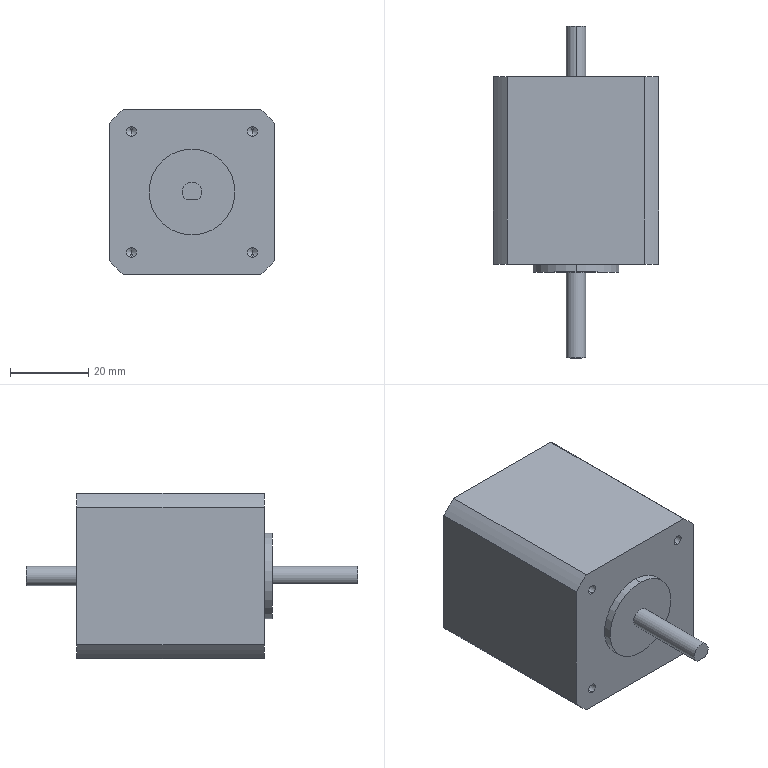Part | NX | features BREP 1 | 1 solid | 35 faces | box 42.3 x 85 x 42.3 mm | volume 86047 mm3 | cylinder 17 | plane 10 | cone 8 | commonest cylinder face diameters 2.5 x8 55 x4 5 x3 22 x2
STEP:
#1=CARTESIAN_POINT('',(1.5,0.,-2.));
#2=VERTEX_POINT('',#1);
#3=CARTESIAN_POINT('',(-1.5,0.,-2.));
#4=VERTEX_POINT('',#3);
#5=CARTESIAN_POINT('',(1.5,0.,-2.));
#6=DIRECTION('',(-1.,0.,0.));
#7=VECTOR('',#6,1000.);
#8=LINE('',#5,#7);
#9=EDGE_CURVE('',#2,#4,#8,.T.);
#10=ORIENTED_EDGE('',*,*,#9,.T.);
#11=CARTESIAN_POINT('',(-1.5,22.,-2.));
#12=VERTEX_POINT('',#11);
#13=CARTESIAN_POINT('',(-1.5,22.,-2.));
#14=DIRECTION('',(0.,-1.,0.));
#15=VECTOR('',#14,1000.);
#16=LINE('',#13,#15);
#17=EDGE_CURVE('',#4,#12,#16,.F.);
#18=ORIENTED_EDGE('',*,*,#17,.T.);
#19=CARTESIAN_POINT('',(1.5,22.,-2.));
#20=VERTEX_POINT('',#19);
#21=CARTESIAN_POINT('',(1.5,22.,-2.));
#22=DIRECTION('',(-1.,0.,0.));
#23=VECTOR('',#22,1000.);
#24=LINE('',#21,#23);
#25=EDGE_CURVE('',#20,#12,#24,.T.);
#26=ORIENTED_EDGE('',*,*,#25,.F.);
#27=CARTESIAN_POINT('',(1.5,22.,-2.));
#28=DIRECTION('',(0.,-1.,0.));
#29=VECTOR('',#28,1000.);
#30=LINE('',#27,#29);
#31=EDGE_CURVE('',#2,#20,#30,.F.);
#32=ORIENTED_EDGE('',*,*,#31,.F.);
#33=EDGE_LOOP('',(#10,#18,#26,#32));
#34=FACE_BOUND('',#33,.T.);
#35=CARTESIAN_POINT('',(1.5,22.,-2.));
#36=DIRECTION('',(0.,0.,1.));
#37=DIRECTION('',(1.,0.,0.));
#38=AXIS2_PLACEMENT_3D('',#35,#36,#37);
#39=PLANE('',#38);
#40=ADVANCED_FACE('',(#34),#39,.F.);
#41=CARTESIAN_POINT('',(-15.5,29.5,-14.25));
#42=VERTEX_POINT('',#41);
#43=CARTESIAN_POINT('',(-15.5,24.,-14.25));
#44=VERTEX_POINT('',#43);
#45=CARTESIAN_POINT('',(-15.5,24.,-14.25));
#46=DIRECTION('',(0.,-1.,0.));
#47=VECTOR('',#46,1000.);
#48=LINE('',#45,#47);
#49=EDGE_CURVE('',#42,#44,#48,.T.);
#50=ORIENTED_EDGE('',*,*,#49,.F.);
#51=CARTESIAN_POINT('',(-15.5,29.5,-16.75));
#52=VERTEX_POINT('',#51);
#53=CARTESIAN_POINT('',(-15.5,29.5,-15.5));
#54=DIRECTION('',(0.,-1.,0.));
#55=DIRECTION('',(0.,0.,-1.));
#56=AXIS2_PLACEMENT_3D('',#53,#54,#55);
#57=CIRCLE('',#56,1.25);
#58=EDGE_CURVE('',#52,#42,#57,.T.);
#59=ORIENTED_EDGE('',*,*,#58,.F.);
#60=CARTESIAN_POINT('',(-15.5,24.,-16.75));
#61=VERTEX_POINT('',#60);
#62=CARTESIAN_POINT('',(-15.5,24.,-16.75));
#63=DIRECTION('',(0.,-1.,0.));
#64=VECTOR('',#63,1000.);
#65=LINE('',#62,#64);
#66=EDGE_CURVE('',#52,#61,#65,.T.);
#67=ORIENTED_EDGE('',*,*,#66,.T.);
#68=CARTESIAN_POINT('',(-15.5,24.,-15.5));
#69=DIRECTION('',(0.,-1.,0.));
#70=DIRECTION('',(0.,0.,-1.));
#71=AXIS2_PLACEMENT_3D('',#68,#69,#70);
#72=CIRCLE('',#71,1.25);
#73=EDGE_CURVE('',#61,#44,#72,.T.);
#74=ORIENTED_EDGE('',*,*,#73,.T.);
#75=EDGE_LOOP('',(#50,#59,#67,#74));
#76=FACE_BOUND('',#75,.T.);
#77=CARTESIAN_POINT('',(-15.5,24.,-15.5));
#78=DIRECTION('',(0.,-1.,0.));
#79=DIRECTION('',(0.,0.,-1.));
#80=AXIS2_PLACEMENT_3D('',#77,#78,#79);
#81=CYLINDRICAL_SURFACE('',#80,1.25);
#82=ADVANCED_FACE('',(#76),#81,.F.);
#83=CARTESIAN_POINT('',(-15.5,30.251,-15.5));
#84=VERTEX_POINT('',#83);
#85=CARTESIAN_POINT('',(-15.5,29.5,-14.25));
#86=DIRECTION('',(0.,-0.515,0.8572));
#87=VECTOR('',#86,1000.);
#88=LINE('',#85,#87);
#89=EDGE_CURVE('',#42,#84,#88,.F.);
#90=ORIENTED_EDGE('',*,*,#89,.T.);
#91=CARTESIAN_POINT('',(-15.5,29.5,-16.75));
#92=DIRECTION('',(0.,-0.515,-0.8572));
#93=VECTOR('',#92,1000.);
#94=LINE('',#91,#93);
#95=EDGE_CURVE('',#52,#84,#94,.F.);
#96=ORIENTED_EDGE('',*,*,#95,.F.);
#97=ORIENTED_EDGE('',*,*,#58,.T.);
#98=EDGE_LOOP('',(#90,#96,#97));
#99=FACE_BOUND('',#98,.T.);
#100=CARTESIAN_POINT('',(-15.5,29.5,-15.5));
#101=DIRECTION('',(0.,-1.,0.));
#102=DIRECTION('',(0.,0.,-1.));
#103=AXIS2_PLACEMENT_3D('',#100,#101,#102);
#104=CONICAL_SURFACE('',#103,1.25,1.03);
#105=ADVANCED_FACE('',(#99),#104,.F.);
#106=CARTESIAN_POINT('',(15.5,29.5,16.75));
#107=VERTEX_POINT('',#106);
#108=CARTESIAN_POINT('',(15.5,24.,16.75));
#109=VERTEX_POINT('',#108);
#110=CARTESIAN_POINT('',(15.5,24.,16.75));
#111=DIRECTION('',(0.,-1.,0.));
#112=VECTOR('',#111,1000.);
#113=LINE('',#110,#112);
#114=EDGE_CURVE('',#107,#109,#113,.T.);
#115=ORIENTED_EDGE('',*,*,#114,.F.);
#116=CARTESIAN_POINT('',(15.5,29.5,14.25));
#117=VERTEX_POINT('',#116);
#118=CARTESIAN_POINT('',(15.5,29.5,15.5));
#119=DIRECTION('',(0.,-1.,0.));
#120=DIRECTION('',(0.,0.,-1.));
#121=AXIS2_PLACEMENT_3D('',#118,#119,#120);
#122=CIRCLE('',#121,1.25);
#123=EDGE_CURVE('',#117,#107,#122,.T.);
#124=ORIENTED_EDGE('',*,*,#123,.F.);
#125=CARTESIAN_POINT('',(15.5,24.,14.25));
#126=VERTEX_POINT('',#125);
#127=CARTESIAN_POINT('',(15.5,24.,14.25));
#128=DIRECTION('',(0.,-1.,0.));
#129=VECTOR('',#128,1000.);
#130=LINE('',#127,#129);
#131=EDGE_CURVE('',#117,#126,#130,.T.);
#132=ORIENTED_EDGE('',*,*,#131,.T.);
#133=CARTESIAN_POINT('',(15.5,24.,15.5));
#134=DIRECTION('',(0.,-1.,0.));
#135=DIRECTION('',(0.,0.,-1.));
#136=AXIS2_PLACEMENT_3D('',#133,#134,#135);
#137=CIRCLE('',#136,1.25);
#138=EDGE_CURVE('',#126,#109,#137,.T.);
#139=ORIENTED_EDGE('',*,*,#138,.T.);
#140=EDGE_LOOP('',(#115,#124,#132,#139));
#141=FACE_BOUND('',#140,.T.);
#142=CARTESIAN_POINT('',(15.5,24.,15.5));
#143=DIRECTION('',(0.,-1.,0.));
#144=DIRECTION('',(0.,0.,-1.));
#145=AXIS2_PLACEMENT_3D('',#142,#143,#144);
#146=CYLINDRICAL_SURFACE('',#145,1.25);
#147=ADVANCED_FACE('',(#141),#146,.F.);
#148=CARTESIAN_POINT('',(15.5,30.251,15.5));
#149=VERTEX_POINT('',#148);
#150=CARTESIAN_POINT('',(15.5,29.5,16.75));
#151=DIRECTION('',(0.,-0.515,0.8572));
#152=VECTOR('',#151,1000.);
#153=LINE('',#150,#152);
#154=EDGE_CURVE('',#107,#149,#153,.F.);
#155=ORIENTED_EDGE('',*,*,#154,.T.);
#156=CARTESIAN_POINT('',(15.5,29.5,14.25));
#157=DIRECTION('',(0.,-0.515,-0.8572));
#158=VECTOR('',#157,1000.);
#159=LINE('',#156,#158);
#160=EDGE_CURVE('',#117,#149,#159,.F.);
#161=ORIENTED_EDGE('',*,*,#160,.F.);
#162=ORIENTED_EDGE('',*,*,#123,.T.);
#163=EDGE_LOOP('',(#155,#161,#162));
#164=FACE_BOUND('',#163,.T.);
#165=CARTESIAN_POINT('',(15.5,29.5,15.5));
#166=DIRECTION('',(0.,-1.,0.));
#167=DIRECTION('',(0.,0.,-1.));
#168=AXIS2_PLACEMENT_3D('',#165,#166,#167);
#169=CONICAL_SURFACE('',#168,1.25,1.03);
#170=ADVANCED_FACE('',(#164),#169,.F.);
#171=CARTESIAN_POINT('',(15.5,29.5,-14.25));
#172=VERTEX_POINT('',#171);
#173=CARTESIAN_POINT('',(15.5,24.,-14.25));
#174=VERTEX_POINT('',#173);
#175=CARTESIAN_POINT('',(15.5,24.,-14.25));
#176=DIRECTION('',(0.,-1.,0.));
#177=VECTOR('',#176,1000.);
#178=LINE('',#175,#177);
#179=EDGE_CURVE('',#172,#174,#178,.T.);
#180=ORIENTED_EDGE('',*,*,#179,.F.);
#181=CARTESIAN_POINT('',(15.5,29.5,-16.75));
#182=VERTEX_POINT('',#181);
#183=CARTESIAN_POINT('',(15.5,29.5,-15.5));
#184=DIRECTION('',(0.,-1.,0.));
#185=DIRECTION('',(0.,0.,-1.));
#186=AXIS2_PLACEMENT_3D('',#183,#184,#185);
#187=CIRCLE('',#186,1.25);
#188=EDGE_CURVE('',#182,#172,#187,.T.);
#189=ORIENTED_EDGE('',*,*,#188,.F.);
#190=CARTESIAN_POINT('',(15.5,24.,-16.75));
#191=VERTEX_POINT('',#190);
#192=CARTESIAN_POINT('',(15.5,24.,-16.75));
#193=DIRECTION('',(0.,-1.,0.));
#194=VECTOR('',#193,1000.);
#195=LINE('',#192,#194);
#196=EDGE_CURVE('',#182,#191,#195,.T.);
#197=ORIENTED_EDGE('',*,*,#196,.T.);
#198=CARTESIAN_POINT('',(15.5,24.,-15.5));
#199=DIRECTION('',(0.,-1.,0.));
#200=DIRECTION('',(0.,0.,-1.));
#201=AXIS2_PLACEMENT_3D('',#198,#199,#200);
#202=CIRCLE('',#201,1.25);
#203=EDGE_CURVE('',#191,#174,#202,.T.);
#204=ORIENTED_EDGE('',*,*,#203,.T.);
#205=EDGE_LOOP('',(#180,#189,#197,#204));
#206=FACE_BOUND('',#205,.T.);
#207=CARTESIAN_POINT('',(15.5,24.,-15.5));
#208=DIRECTION('',(0.,-1.,0.));
#209=DIRECTION('',(0.,0.,-1.));
#210=AXIS2_PLACEMENT_3D('',#207,#208,#209);
#211=CYLINDRICAL_SURFACE('',#210,1.25);
#212=ADVANCED_FACE('',(#206),#211,.F.);
#213=CARTESIAN_POINT('',(15.5,30.251,-15.5));
#214=VERTEX_POINT('',#213);
#215=CARTESIAN_POINT('',(15.5,29.5,-14.25));
#216=DIRECTION('',(0.,-0.515,0.8572));
#217=VECTOR('',#216,1000.);
#218=LINE('',#215,#217);
#219=EDGE_CURVE('',#172,#214,#218,.F.);
#220=ORIENTED_EDGE('',*,*,#219,.T.);
#221=CARTESIAN_POINT('',(15.5,29.5,-16.75));
#222=DIRECTION('',(0.,-0.515,-0.8572));
#223=VECTOR('',#222,1000.);
#224=LINE('',#221,#223);
#225=EDGE_CURVE('',#182,#214,#224,.F.);
#226=ORIENTED_EDGE('',*,*,#225,.F.);
#227=ORIENTED_EDGE('',*,*,#188,.T.);
#228=EDGE_LOOP('',(#220,#226,#227));
#229=FACE_BOUND('',#228,.T.);
#230=CARTESIAN_POINT('',(15.5,29.5,-15.5));
#231=DIRECTION('',(0.,-1.,0.));
#232=DIRECTION('',(0.,0.,-1.));
#233=AXIS2_PLACEMENT_3D('',#230,#231,#232);
#234=CONICAL_SURFACE('',#233,1.25,1.03);
#235=ADVANCED_FACE('',(#229),#234,.F.);
#236=CARTESIAN_POINT('',(-15.5,29.5,16.75));
#237=VERTEX_POINT('',#236);
#238=CARTESIAN_POINT('',(-15.5,24.,16.75));
#239=VERTEX_POINT('',#238);
#240=CARTESIAN_POINT('',(-15.5,24.,16.75));
#241=DIRECTION('',(0.,-1.,0.));
#242=VECTOR('',#241,1000.);
#243=LINE('',#240,#242);
#244=EDGE_CURVE('',#237,#239,#243,.T.);
#245=ORIENTED_EDGE('',*,*,#244,.F.);
#246=CARTESIAN_POINT('',(-15.5,29.5,14.25));
#247=VERTEX_POINT('',#246);
#248=CARTESIAN_POINT('',(-15.5,29.5,15.5));
#249=DIRECTION('',(0.,-1.,0.));
#250=DIRECTION('',(0.,0.,-1.));
#251=AXIS2_PLACEMENT_3D('',#248,#249,#250);
#252=CIRCLE('',#251,1.25);
#253=EDGE_CURVE('',#247,#237,#252,.T.);
#254=ORIENTED_EDGE('',*,*,#253,.F.);
#255=CARTESIAN_POINT('',(-15.5,24.,14.25));
#256=VERTEX_POINT('',#255);
#257=CARTESIAN_POINT('',(-15.5,24.,14.25));
#258=DIRECTION('',(0.,-1.,0.));
#259=VECTOR('',#258,1000.);
#260=LINE('',#257,#259);
#261=EDGE_CURVE('',#247,#256,#260,.T.);
#262=ORIENTED_EDGE('',*,*,#261,.T.);
#263=CARTESIAN_POINT('',(-15.5,24.,15.5));
#264=DIRECTION('',(0.,-1.,0.));
#265=DIRECTION('',(0.,0.,-1.));
#266=AXIS2_PLACEMENT_3D('',#263,#264,#265);
#267=CIRCLE('',#266,1.25);
#268=EDGE_CURVE('',#256,#239,#267,.T.);
#269=ORIENTED_EDGE('',*,*,#268,.T.);
#270=EDGE_LOOP('',(#245,#254,#262,#269));
#271=FACE_BOUND('',#270,.T.);
#272=CARTESIAN_POINT('',(-15.5,24.,15.5));
#273=DIRECTION('',(0.,-1.,0.));
#274=DIRECTION('',(0.,0.,-1.));
#275=AXIS2_PLACEMENT_3D('',#272,#273,#274);
#276=CYLINDRICAL_SURFACE('',#275,1.25);
#277=ADVANCED_FACE('',(#271),#276,.F.);
#278=CARTESIAN_POINT('',(-15.5,30.251,15.5));
#279=VERTEX_POINT('',#278);
#280=CARTESIAN_POINT('',(-15.5,29.5,16.75));
#281=DIRECTION('',(0.,-0.515,0.8572));
#282=VECTOR('',#281,1000.);
#283=LINE('',#280,#282);
#284=EDGE_CURVE('',#237,#279,#283,.F.);
#285=ORIENTED_EDGE('',*,*,#284,.T.);
#286=CARTESIAN_POINT('',(-15.5,29.5,14.25));
#287=DIRECTION('',(0.,-0.515,-0.8572));
#288=VECTOR('',#287,1000.);
#289=LINE('',#286,#288);
#290=EDGE_CURVE('',#247,#279,#289,.F.);
#291=ORIENTED_EDGE('',*,*,#290,.F.);
#292=ORIENTED_EDGE('',*,*,#253,.T.);
#293=EDGE_LOOP('',(#285,#291,#292));
#294=FACE_BOUND('',#293,.T.);
#295=CARTESIAN_POINT('',(-15.5,29.5,15.5));
#296=DIRECTION('',(0.,-1.,0.));
#297=DIRECTION('',(0.,0.,-1.));
#298=AXIS2_PLACEMENT_3D('',#295,#296,#297);
#299=CONICAL_SURFACE('',#298,1.25,1.03);
#300=ADVANCED_FACE('',(#294),#299,.F.);
#301=CARTESIAN_POINT('',(-21.15,72.,-17.576));
#302=VERTEX_POINT('',#301);
#303=CARTESIAN_POINT('',(-21.15,24.,-17.576));
#304=VERTEX_POINT('',#303);
#305=CARTESIAN_POINT('',(-21.15,0.,-17.576));
#306=DIRECTION('',(0.,-1.,0.));
#307=VECTOR('',#306,1000.);
#308=LINE('',#305,#307);
#309=EDGE_CURVE('',#302,#304,#308,.T.);
#310=ORIENTED_EDGE('',*,*,#309,.T.);
#311=CARTESIAN_POINT('',(-21.15,24.,17.576));
#312=VERTEX_POINT('',#311);
#313=CARTESIAN_POINT('',(-21.15,24.,0.));
#314=DIRECTION('',(0.,0.,1.));
#315=VECTOR('',#314,1000.);
#316=LINE('',#313,#315);
#317=EDGE_CURVE('',#304,#312,#316,.T.);
#318=ORIENTED_EDGE('',*,*,#317,.T.);
#319=CARTESIAN_POINT('',(-21.15,72.,17.576));
#320=VERTEX_POINT('',#319);
#321=CARTESIAN_POINT('',(-21.15,0.,17.576));
#322=DIRECTION('',(0.,1.,0.));
#323=VECTOR('',#322,1000.);
#324=LINE('',#321,#323);
#325=EDGE_CURVE('',#312,#320,#324,.T.);
#326=ORIENTED_EDGE('',*,*,#325,.T.);
#327=CARTESIAN_POINT('',(-21.15,72.,0.));
#328=DIRECTION('',(0.,0.,-1.));
#329=VECTOR('',#328,1000.);
#330=LINE('',#327,#329);
#331=EDGE_CURVE('',#320,#302,#330,.T.);
#332=ORIENTED_EDGE('',*,*,#331,.T.);
#333=EDGE_LOOP('',(#310,#318,#326,#332));
#334=FACE_BOUND('',#333,.T.);
#335=CARTESIAN_POINT('',(-21.15,0.,-21.15));
#336=DIRECTION('',(-1.,0.,0.));
#337=DIRECTION('',(0.,0.,1.));
#338=AXIS2_PLACEMENT_3D('',#335,#336,#337);
#339=PLANE('',#338);
#340=ADVANCED_FACE('',(#334),#339,.T.);
#341=CARTESIAN_POINT('',(17.576,72.,-21.15));
#342=VERTEX_POINT('',#341);
#343=CARTESIAN_POINT('',(17.576,24.,-21.15));
#344=VERTEX_POINT('',#343);
#345=CARTESIAN_POINT('',(17.576,0.,-21.15));
#346=DIRECTION('',(0.,-1.,0.));
#347=VECTOR('',#346,1000.);
#348=LINE('',#345,#347);
#349=EDGE_CURVE('',#342,#344,#348,.T.);
#350=ORIENTED_EDGE('',*,*,#349,.T.);
#351=CARTESIAN_POINT('',(-17.576,24.,-21.15));
#352=VERTEX_POINT('',#351);
#353=CARTESIAN_POINT('',(-11.,24.,-21.15));
#354=DIRECTION('',(-1.,0.,0.));
#355=VECTOR('',#354,1000.);
#356=LINE('',#353,#355);
#357=EDGE_CURVE('',#344,#352,#356,.T.);
#358=ORIENTED_EDGE('',*,*,#357,.T.);
#359=CARTESIAN_POINT('',(-17.576,72.,-21.15));
#360=VERTEX_POINT('',#359);
#361=CARTESIAN_POINT('',(-17.576,0.,-21.15));
#362=DIRECTION('',(0.,1.,0.));
#363=VECTOR('',#362,1000.);
#364=LINE('',#361,#363);
#365=EDGE_CURVE('',#352,#360,#364,.T.);
#366=ORIENTED_EDGE('',*,*,#365,.T.);
#367=CARTESIAN_POINT('',(-27.5,72.,-21.15));
#368=DIRECTION('',(1.,0.,0.));
#369=VECTOR('',#368,1000.);
#370=LINE('',#367,#369);
#371=EDGE_CURVE('',#360,#342,#370,.T.);
#372=ORIENTED_EDGE('',*,*,#371,.T.);
#373=EDGE_LOOP('',(#350,#358,#366,#372));
#374=FACE_BOUND('',#373,.T.);
#375=CARTESIAN_POINT('',(21.15,0.,-21.15));
#376=DIRECTION('',(0.,0.,-1.));
#377=DIRECTION('',(-1.,0.,0.));
#378=AXIS2_PLACEMENT_3D('',#375,#376,#377);
#379=PLANE('',#378);
#380=ADVANCED_FACE('',(#374),#379,.T.);
#381=CARTESIAN_POINT('',(21.15,72.,17.576));
#382=VERTEX_POINT('',#381);
#383=CARTESIAN_POINT('',(21.15,24.,17.576));
#384=VERTEX_POINT('',#383);
#385=CARTESIAN_POINT('',(21.15,0.,17.576));
#386=DIRECTION('',(0.,-1.,0.));
#387=VECTOR('',#386,1000.);
#388=LINE('',#385,#387);
#389=EDGE_CURVE('',#382,#384,#388,.T.);
#390=ORIENTED_EDGE('',*,*,#389,.T.);
#391=CARTESIAN_POINT('',(21.15,24.,-17.576));
#392=VERTEX_POINT('',#391);
#393=CARTESIAN_POINT('',(21.15,24.,0.));
#394=DIRECTION('',(0.,0.,-1.));
#395=VECTOR('',#394,1000.);
#396=LINE('',#393,#395);
#397=EDGE_CURVE('',#384,#392,#396,.T.);
#398=ORIENTED_EDGE('',*,*,#397,.T.);
#399=CARTESIAN_POINT('',(21.15,72.,-17.576));
#400=VERTEX_POINT('',#399);
#401=CARTESIAN_POINT('',(21.15,0.,-17.576));
#402=DIRECTION('',(0.,1.,0.));
#403=VECTOR('',#402,1000.);
#404=LINE('',#401,#403);
#405=EDGE_CURVE('',#392,#400,#404,.T.);
#406=ORIENTED_EDGE('',*,*,#405,.T.);
#407=CARTESIAN_POINT('',(21.15,72.,0.));
#408=DIRECTION('',(0.,0.,1.));
#409=VECTOR('',#408,1000.);
#410=LINE('',#407,#409);
#411=EDGE_CURVE('',#400,#382,#410,.T.);
#412=ORIENTED_EDGE('',*,*,#411,.T.);
#413=EDGE_LOOP('',(#390,#398,#406,#412));
#414=FACE_BOUND('',#413,.T.);
#415=CARTESIAN_POINT('',(21.15,0.,-21.15));
#416=DIRECTION('',(1.,0.,0.));
#417=DIRECTION('',(0.,0.,-1.));
#418=AXIS2_PLACEMENT_3D('',#415,#416,#417);
#419=PLANE('',#418);
#420=ADVANCED_FACE('',(#414),#419,.T.);
#421=CARTESIAN_POINT('',(-17.576,72.,21.15));
#422=VERTEX_POINT('',#421);
#423=CARTESIAN_POINT('',(-17.576,24.,21.15));
#424=VERTEX_POINT('',#423);
#425=CARTESIAN_POINT('',(-17.576,0.,21.15));
#426=DIRECTION('',(0.,-1.,0.));
#427=VECTOR('',#426,1000.);
#428=LINE('',#425,#427);
#429=EDGE_CURVE('',#422,#424,#428,.T.);
#430=ORIENTED_EDGE('',*,*,#429,.T.);
#431=CARTESIAN_POINT('',(17.576,24.,21.15));
#432=VERTEX_POINT('',#431);
#433=CARTESIAN_POINT('',(-11.,24.,21.15));
#434=DIRECTION('',(1.,0.,0.));
#435=VECTOR('',#434,1000.);
#436=LINE('',#433,#435);
#437=EDGE_CURVE('',#424,#432,#436,.T.);
#438=ORIENTED_EDGE('',*,*,#437,.T.);
#439=CARTESIAN_POINT('',(17.576,72.,21.15));
#440=VERTEX_POINT('',#439);
#441=CARTESIAN_POINT('',(17.576,0.,21.15));
#442=DIRECTION('',(0.,1.,0.));
#443=VECTOR('',#442,1000.);
#444=LINE('',#441,#443);
#445=EDGE_CURVE('',#432,#440,#444,.T.);
#446=ORIENTED_EDGE('',*,*,#445,.T.);
#447=CARTESIAN_POINT('',(-27.5,72.,21.15));
#448=DIRECTION('',(-1.,0.,0.));
#449=VECTOR('',#448,1000.);
#450=LINE('',#447,#449);
#451=EDGE_CURVE('',#440,#422,#450,.T.);
#452=ORIENTED_EDGE('',*,*,#451,.T.);
#453=EDGE_LOOP('',(#430,#438,#446,#452));
#454=FACE_BOUND('',#453,.T.);
#455=CARTESIAN_POINT('',(21.15,0.,21.15));
#456=DIRECTION('',(0.,0.,1.));
#457=DIRECTION('',(1.,0.,0.));
#458=AXIS2_PLACEMENT_3D('',#455,#456,#457);
#459=PLANE('',#458);
#460=ADVANCED_FACE('',(#454),#459,.T.);
#461=CARTESIAN_POINT('',(0.,85.,-2.5));
#462=VERTEX_POINT('',#461);
#463=CARTESIAN_POINT('',(0.,85.,2.5));
#464=VERTEX_POINT('',#463);
#465=CARTESIAN_POINT('',(0.,85.,0.));
#466=DIRECTION('',(0.,-1.,0.));
#467=DIRECTION('',(0.,0.,-1.));
#468=AXIS2_PLACEMENT_3D('',#465,#466,#467);
#469=CIRCLE('',#468,2.5);
#470=EDGE_CURVE('',#462,#464,#469,.T.);
#471=ORIENTED_EDGE('',*,*,#470,.F.);
#472=CARTESIAN_POINT('',(0.,85.,0.));
#473=DIRECTION('',(0.,-1.,0.));
#474=DIRECTION('',(0.,0.,-1.));
#475=AXIS2_PLACEMENT_3D('',#472,#473,#474);
#476=CIRCLE('',#475,2.5);
#477=EDGE_CURVE('',#464,#462,#476,.T.);
#478=ORIENTED_EDGE('',*,*,#477,.F.);
#479=EDGE_LOOP('',(#471,#478));
#480=FACE_BOUND('',#479,.T.);
#481=CARTESIAN_POINT('',(-2.5,85.,0.));
#482=DIRECTION('',(0.,-1.,0.));
#483=DIRECTION('',(0.,0.,-1.));
#484=AXIS2_PLACEMENT_3D('',#481,#482,#483);
#485=PLANE('',#484);
#486=ADVANCED_FACE('',(#480),#485,.F.);
#487=CARTESIAN_POINT('',(0.,72.,2.5));
#488=VERTEX_POINT('',#487);
#489=CARTESIAN_POINT('',(0.,0.,2.5));
#490=DIRECTION('',(0.,-1.,0.));
#491=VECTOR('',#490,1000.);
#492=LINE('',#489,#491);
#493=EDGE_CURVE('',#464,#488,#492,.T.);
#494=ORIENTED_EDGE('',*,*,#493,.F.);
#495=ORIENTED_EDGE('',*,*,#477,.T.);
#496=CARTESIAN_POINT('',(0.,72.,-2.5));
#497=VERTEX_POINT('',#496);
#498=CARTESIAN_POINT('',(0.,0.,-2.5));
#499=DIRECTION('',(0.,-1.,0.));
#500=VECTOR('',#499,1000.);
#501=LINE('',#498,#500);
#502=EDGE_CURVE('',#462,#497,#501,.T.);
#503=ORIENTED_EDGE('',*,*,#502,.T.);
#504=CARTESIAN_POINT('',(0.,72.,0.));
#505=DIRECTION('',(0.,-1.,0.));
#506=DIRECTION('',(0.,0.,-1.));
#507=AXIS2_PLACEMENT_3D('',#504,#505,#506);
#508=CIRCLE('',#507,2.5);
#509=EDGE_CURVE('',#488,#497,#508,.T.);
#510=ORIENTED_EDGE('',*,*,#509,.F.);
#511=EDGE_LOOP('',(#494,#495,#503,#510));
#512=FACE_BOUND('',#511,.T.);
#513=CARTESIAN_POINT('',(0.,0.,0.));
#514=DIRECTION('',(0.,-1.,0.));
#515=DIRECTION('',(0.,0.,-1.));
#516=AXIS2_PLACEMENT_3D('',#513,#514,#515);
#517=CYLINDRICAL_SURFACE('',#516,2.5);
#518=ADVANCED_FACE('',(#512),#517,.T.);
#519=CARTESIAN_POINT('',(0.,24.,11.));
#520=VERTEX_POINT('',#519);
#521=CARTESIAN_POINT('',(0.,22.,11.));
#522=VERTEX_POINT('',#521);
#523=CARTESIAN_POINT('',(0.,0.,11.));
#524=DIRECTION('',(0.,-1.,0.));
#525=VECTOR('',#524,1000.);
#526=LINE('',#523,#525);
#527=EDGE_CURVE('',#520,#522,#526,.T.);
#528=ORIENTED_EDGE('',*,*,#527,.F.);
#529=CARTESIAN_POINT('',(0.,24.,-11.));
#530=VERTEX_POINT('',#529);
#531=CARTESIAN_POINT('',(0.,24.,0.));
#532=DIRECTION('',(0.,-1.,0.));
#533=DIRECTION('',(0.,0.,-1.));
#534=AXIS2_PLACEMENT_3D('',#531,#532,#533);
#535=CIRCLE('',#534,11.);
#536=EDGE_CURVE('',#520,#530,#535,.T.);
#537=ORIENTED_EDGE('',*,*,#536,.T.);
#538=CARTESIAN_POINT('',(0.,22.,-11.));
#539=VERTEX_POINT('',#538);
#540=CARTESIAN_POINT('',(0.,0.,-11.));
#541=DIRECTION('',(0.,-1.,0.));
#542=VECTOR('',#541,1000.);
#543=LINE('',#540,#542);
#544=EDGE_CURVE('',#530,#539,#543,.T.);
#545=ORIENTED_EDGE('',*,*,#544,.T.);
#546=CARTESIAN_POINT('',(0.,22.,0.));
#547=DIRECTION('',(0.,-1.,0.));
#548=DIRECTION('',(0.,0.,-1.));
#549=AXIS2_PLACEMENT_3D('',#546,#547,#548);
#550=CIRCLE('',#549,11.);
#551=EDGE_CURVE('',#522,#539,#550,.T.);
#552=ORIENTED_EDGE('',*,*,#551,.F.);
#553=EDGE_LOOP('',(#528,#537,#545,#552));
#554=FACE_BOUND('',#553,.T.);
#555=CARTESIAN_POINT('',(0.,0.,0.));
#556=DIRECTION('',(0.,-1.,0.));
#557=DIRECTION('',(0.,0.,-1.));
#558=AXIS2_PLACEMENT_3D('',#555,#556,#557);
#559=CYLINDRICAL_SURFACE('',#558,11.);
#560=ADVANCED_FACE('',(#554),#559,.T.);
#561=CARTESIAN_POINT('',(0.,22.,0.));
#562=DIRECTION('',(0.,-1.,0.));
#563=DIRECTION('',(0.,0.,-1.));
#564=AXIS2_PLACEMENT_3D('',#561,#562,#563);
#565=CIRCLE('',#564,11.);
#566=EDGE_CURVE('',#539,#522,#565,.T.);
#567=ORIENTED_EDGE('',*,*,#566,.T.);
#568=ORIENTED_EDGE('',*,*,#551,.T.);
#569=EDGE_LOOP('',(#567,#568));
#570=FACE_BOUND('',#569,.T.);
#571=CARTESIAN_POINT('',(0.,22.,0.));
#572=DIRECTION('',(0.,-1.,0.));
#573=DIRECTION('',(0.,0.,-1.));
#574=AXIS2_PLACEMENT_3D('',#571,#572,#573);
#575=CIRCLE('',#574,2.5);
#576=EDGE_CURVE('',#20,#12,#575,.T.);
#577=ORIENTED_EDGE('',*,*,#576,.F.);
#578=ORIENTED_EDGE('',*,*,#25,.T.);
#579=EDGE_LOOP('',(#577,#578));
#580=FACE_BOUND('',#579,.T.);
#581=CARTESIAN_POINT('',(-2.5,22.,0.));
#582=DIRECTION('',(0.,1.,0.));
#583=DIRECTION('',(0.,0.,1.));
#584=AXIS2_PLACEMENT_3D('',#581,#582,#583);
#585=PLANE('',#584);
#586=ADVANCED_FACE('',(#570,#580),#585,.F.);
#587=ORIENTED_EDGE('',*,*,#576,.T.);
#588=ORIENTED_EDGE('',*,*,#17,.F.);
#589=CARTESIAN_POINT('',(0.,0.,0.));
#590=DIRECTION('',(0.,-1.,0.));
#591=DIRECTION('',(0.,0.,-1.));
#592=AXIS2_PLACEMENT_3D('',#589,#590,#591);
#593=CIRCLE('',#592,2.5);
#594=EDGE_CURVE('',#2,#4,#593,.T.);
#595=ORIENTED_EDGE('',*,*,#594,.F.);
#596=ORIENTED_EDGE('',*,*,#31,.T.);
#597=EDGE_LOOP('',(#587,#588,#595,#596));
#598=FACE_BOUND('',#597,.T.);
#599=CARTESIAN_POINT('',(0.,0.,0.));
#600=DIRECTION('',(0.,-1.,0.));
#601=DIRECTION('',(0.,0.,-1.));
#602=AXIS2_PLACEMENT_3D('',#599,#600,#601);
#603=CYLINDRICAL_SURFACE('',#602,2.5);
#604=ADVANCED_FACE('',(#598),#603,.T.);
#605=ORIENTED_EDGE('',*,*,#594,.T.);
#606=ORIENTED_EDGE('',*,*,#9,.F.);
#607=EDGE_LOOP('',(#605,#606));
#608=FACE_BOUND('',#607,.T.);
#609=CARTESIAN_POINT('',(0.,0.,0.));
#610=DIRECTION('',(0.,1.,0.));
#611=DIRECTION('',(0.,0.,1.));
#612=AXIS2_PLACEMENT_3D('',#609,#610,#611);
#613=PLANE('',#612);
#614=ADVANCED_FACE('',(#608),#613,.F.);
#615=ORIENTED_EDGE('',*,*,#331,.F.);
#616=CARTESIAN_POINT('',(0.,72.,0.));
#617=DIRECTION('',(0.,-1.,0.));
#618=DIRECTION('',(0.,0.,-1.));
#619=AXIS2_PLACEMENT_3D('',#616,#617,#618);
#620=CIRCLE('',#619,27.5);
#621=EDGE_CURVE('',#422,#320,#620,.T.);
#622=ORIENTED_EDGE('',*,*,#621,.F.);
#623=ORIENTED_EDGE('',*,*,#451,.F.);
#624=CARTESIAN_POINT('',(0.,72.,0.));
#625=DIRECTION('',(0.,-1.,0.));
#626=DIRECTION('',(0.,0.,-1.));
#627=AXIS2_PLACEMENT_3D('',#624,#625,#626);
#628=CIRCLE('',#627,27.5);
#629=EDGE_CURVE('',#382,#440,#628,.T.);
#630=ORIENTED_EDGE('',*,*,#629,.F.);
#631=ORIENTED_EDGE('',*,*,#411,.F.);
#632=CARTESIAN_POINT('',(0.,72.,0.));
#633=DIRECTION('',(0.,-1.,0.));
#634=DIRECTION('',(0.,0.,-1.));
#635=AXIS2_PLACEMENT_3D('',#632,#633,#634);
#636=CIRCLE('',#635,27.5);
#637=EDGE_CURVE('',#342,#400,#636,.T.);
#638=ORIENTED_EDGE('',*,*,#637,.F.);
#639=ORIENTED_EDGE('',*,*,#371,.F.);
#640=CARTESIAN_POINT('',(0.,72.,0.));
#641=DIRECTION('',(0.,-1.,0.));
#642=DIRECTION('',(0.,0.,-1.));
#643=AXIS2_PLACEMENT_3D('',#640,#641,#642);
#644=CIRCLE('',#643,27.5);
#645=EDGE_CURVE('',#302,#360,#644,.T.);
#646=ORIENTED_EDGE('',*,*,#645,.F.);
#647=EDGE_LOOP('',(#615,#622,#623,#630,#631,#638,#639,#646));
#648=FACE_BOUND('',#647,.T.);
#649=CARTESIAN_POINT('',(0.,72.,0.));
#650=DIRECTION('',(0.,-1.,0.));
#651=DIRECTION('',(0.,0.,-1.));
#652=AXIS2_PLACEMENT_3D('',#649,#650,#651);
#653=CIRCLE('',#652,2.5);
#654=EDGE_CURVE('',#497,#488,#653,.T.);
#655=ORIENTED_EDGE('',*,*,#654,.T.);
#656=ORIENTED_EDGE('',*,*,#509,.T.);
#657=EDGE_LOOP('',(#655,#656));
#658=FACE_BOUND('',#657,.T.);
#659=CARTESIAN_POINT('',(-27.5,72.,0.));
#660=DIRECTION('',(0.,-1.,0.));
#661=DIRECTION('',(0.,0.,-1.));
#662=AXIS2_PLACEMENT_3D('',#659,#660,#661);
#663=PLANE('',#662);
#664=ADVANCED_FACE('',(#648,#658),#663,.F.);
#665=ORIENTED_EDGE('',*,*,#389,.F.);
#666=ORIENTED_EDGE('',*,*,#629,.T.);
#667=ORIENTED_EDGE('',*,*,#445,.F.);
#668=CARTESIAN_POINT('',(0.,24.,0.));
#669=DIRECTION('',(0.,-1.,0.));
#670=DIRECTION('',(0.,0.,-1.));
#671=AXIS2_PLACEMENT_3D('',#668,#669,#670);
#672=CIRCLE('',#671,27.5);
#673=EDGE_CURVE('',#384,#432,#672,.T.);
#674=ORIENTED_EDGE('',*,*,#673,.F.);
#675=EDGE_LOOP('',(#665,#666,#667,#674));
#676=FACE_BOUND('',#675,.T.);
#677=CARTESIAN_POINT('',(0.,0.,0.));
#678=DIRECTION('',(0.,-1.,0.));
#679=DIRECTION('',(0.,0.,-1.));
#680=AXIS2_PLACEMENT_3D('',#677,#678,#679);
#681=CYLINDRICAL_SURFACE('',#680,27.5);
#682=ADVANCED_FACE('',(#676),#681,.T.);
#683=ORIENTED_EDGE('',*,*,#349,.F.);
#684=ORIENTED_EDGE('',*,*,#637,.T.);
#685=ORIENTED_EDGE('',*,*,#405,.F.);
#686=CARTESIAN_POINT('',(0.,24.,0.));
#687=DIRECTION('',(0.,-1.,0.));
#688=DIRECTION('',(0.,0.,-1.));
#689=AXIS2_PLACEMENT_3D('',#686,#687,#688);
#690=CIRCLE('',#689,27.5);
#691=EDGE_CURVE('',#344,#392,#690,.T.);
#692=ORIENTED_EDGE('',*,*,#691,.F.);
#693=EDGE_LOOP('',(#683,#684,#685,#692));
#694=FACE_BOUND('',#693,.T.);
#695=CARTESIAN_POINT('',(0.,0.,0.));
#696=DIRECTION('',(0.,-1.,0.));
#697=DIRECTION('',(0.,0.,-1.));
#698=AXIS2_PLACEMENT_3D('',#695,#696,#697);
#699=CYLINDRICAL_SURFACE('',#698,27.5);
#700=ADVANCED_FACE('',(#694),#699,.T.);
#701=ORIENTED_EDGE('',*,*,#325,.F.);
#702=CARTESIAN_POINT('',(0.,24.,0.));
#703=DIRECTION('',(0.,-1.,0.));
#704=DIRECTION('',(0.,0.,-1.));
#705=AXIS2_PLACEMENT_3D('',#702,#703,#704);
#706=CIRCLE('',#705,27.5);
#707=EDGE_CURVE('',#424,#312,#706,.T.);
#708=ORIENTED_EDGE('',*,*,#707,.F.);
#709=ORIENTED_EDGE('',*,*,#429,.F.);
#710=ORIENTED_EDGE('',*,*,#621,.T.);
#711=EDGE_LOOP('',(#701,#708,#709,#710));
#712=FACE_BOUND('',#711,.T.);
#713=CARTESIAN_POINT('',(0.,0.,0.));
#714=DIRECTION('',(0.,-1.,0.));
#715=DIRECTION('',(0.,0.,-1.));
#716=AXIS2_PLACEMENT_3D('',#713,#714,#715);
#717=CYLINDRICAL_SURFACE('',#716,27.5);
#718=ADVANCED_FACE('',(#712),#717,.T.);
#719=ORIENTED_EDGE('',*,*,#309,.F.);
#720=ORIENTED_EDGE('',*,*,#645,.T.);
#721=ORIENTED_EDGE('',*,*,#365,.F.);
#722=CARTESIAN_POINT('',(0.,24.,0.));
#723=DIRECTION('',(0.,-1.,0.));
#724=DIRECTION('',(0.,0.,-1.));
#725=AXIS2_PLACEMENT_3D('',#722,#723,#724);
#726=CIRCLE('',#725,27.5);
#727=EDGE_CURVE('',#304,#352,#726,.T.);
#728=ORIENTED_EDGE('',*,*,#727,.F.);
#729=EDGE_LOOP('',(#719,#720,#721,#728));
#730=FACE_BOUND('',#729,.T.);
#731=CARTESIAN_POINT('',(0.,0.,0.));
#732=DIRECTION('',(0.,-1.,0.));
#733=DIRECTION('',(0.,0.,-1.));
#734=AXIS2_PLACEMENT_3D('',#731,#732,#733);
#735=CYLINDRICAL_SURFACE('',#734,27.5);
#736=ADVANCED_FACE('',(#730),#735,.T.);
#737=ORIENTED_EDGE('',*,*,#317,.F.);
#738=ORIENTED_EDGE('',*,*,#727,.T.);
#739=ORIENTED_EDGE('',*,*,#357,.F.);
#740=ORIENTED_EDGE('',*,*,#691,.T.);
#741=ORIENTED_EDGE('',*,*,#397,.F.);
#742=ORIENTED_EDGE('',*,*,#673,.T.);
#743=ORIENTED_EDGE('',*,*,#437,.F.);
#744=ORIENTED_EDGE('',*,*,#707,.T.);
#745=EDGE_LOOP('',(#737,#738,#739,#740,#741,#742,#743,#744));
#746=FACE_BOUND('',#745,.T.);
#747=CARTESIAN_POINT('',(0.,24.,0.));
#748=DIRECTION('',(0.,-1.,0.));
#749=DIRECTION('',(0.,0.,-1.));
#750=AXIS2_PLACEMENT_3D('',#747,#748,#749);
#751=CIRCLE('',#750,11.);
#752=EDGE_CURVE('',#530,#520,#751,.T.);
#753=ORIENTED_EDGE('',*,*,#752,.F.);
#754=ORIENTED_EDGE('',*,*,#536,.F.);
#755=EDGE_LOOP('',(#753,#754));
#756=FACE_BOUND('',#755,.T.);
#757=ORIENTED_EDGE('',*,*,#268,.F.);
#758=CARTESIAN_POINT('',(-15.5,24.,15.5));
#759=DIRECTION('',(0.,-1.,0.));
#760=DIRECTION('',(0.,0.,-1.));
#761=AXIS2_PLACEMENT_3D('',#758,#759,#760);
#762=CIRCLE('',#761,1.25);
#763=EDGE_CURVE('',#239,#256,#762,.T.);
#764=ORIENTED_EDGE('',*,*,#763,.F.);
#765=EDGE_LOOP('',(#757,#764));
#766=FACE_BOUND('',#765,.T.);
#767=ORIENTED_EDGE('',*,*,#203,.F.);
#768=CARTESIAN_POINT('',(15.5,24.,-15.5));
#769=DIRECTION('',(0.,-1.,0.));
#770=DIRECTION('',(0.,0.,-1.));
#771=AXIS2_PLACEMENT_3D('',#768,#769,#770);
#772=CIRCLE('',#771,1.25);
#773=EDGE_CURVE('',#174,#191,#772,.T.);
#774=ORIENTED_EDGE('',*,*,#773,.F.);
#775=EDGE_LOOP('',(#767,#774));
#776=FACE_BOUND('',#775,.T.);
#777=ORIENTED_EDGE('',*,*,#138,.F.);
#778=CARTESIAN_POINT('',(15.5,24.,15.5));
#779=DIRECTION('',(0.,-1.,0.));
#780=DIRECTION('',(0.,0.,-1.));
#781=AXIS2_PLACEMENT_3D('',#778,#779,#780);
#782=CIRCLE('',#781,1.25);
#783=EDGE_CURVE('',#109,#126,#782,.T.);
#784=ORIENTED_EDGE('',*,*,#783,.F.);
#785=EDGE_LOOP('',(#777,#784));
#786=FACE_BOUND('',#785,.T.);
#787=ORIENTED_EDGE('',*,*,#73,.F.);
#788=CARTESIAN_POINT('',(-15.5,24.,-15.5));
#789=DIRECTION('',(0.,-1.,0.));
#790=DIRECTION('',(0.,0.,-1.));
#791=AXIS2_PLACEMENT_3D('',#788,#789,#790);
#792=CIRCLE('',#791,1.25);
#793=EDGE_CURVE('',#44,#61,#792,.T.);
#794=ORIENTED_EDGE('',*,*,#793,.F.);
#795=EDGE_LOOP('',(#787,#794));
#796=FACE_BOUND('',#795,.T.);
#797=CARTESIAN_POINT('',(-11.,24.,0.));
#798=DIRECTION('',(0.,1.,0.));
#799=DIRECTION('',(0.,0.,1.));
#800=AXIS2_PLACEMENT_3D('',#797,#798,#799);
#801=PLANE('',#800);
#802=ADVANCED_FACE('',(#746,#756,#766,#776,#786,#796),#801,.F.);
#803=ORIENTED_EDGE('',*,*,#752,.T.);
#804=ORIENTED_EDGE('',*,*,#527,.T.);
#805=ORIENTED_EDGE('',*,*,#566,.F.);
#806=ORIENTED_EDGE('',*,*,#544,.F.);
#807=EDGE_LOOP('',(#803,#804,#805,#806));
#808=FACE_BOUND('',#807,.T.);
#809=CARTESIAN_POINT('',(0.,0.,0.));
#810=DIRECTION('',(0.,-1.,0.));
#811=DIRECTION('',(0.,0.,-1.));
#812=AXIS2_PLACEMENT_3D('',#809,#810,#811);
#813=CYLINDRICAL_SURFACE('',#812,11.);
#814=ADVANCED_FACE('',(#808),#813,.T.);
#815=ORIENTED_EDGE('',*,*,#470,.T.);
#816=ORIENTED_EDGE('',*,*,#493,.T.);
#817=ORIENTED_EDGE('',*,*,#654,.F.);
#818=ORIENTED_EDGE('',*,*,#502,.F.);
#819=EDGE_LOOP('',(#815,#816,#817,#818));
#820=FACE_BOUND('',#819,.T.);
#821=CARTESIAN_POINT('',(0.,0.,0.));
#822=DIRECTION('',(0.,-1.,0.));
#823=DIRECTION('',(0.,0.,-1.));
#824=AXIS2_PLACEMENT_3D('',#821,#822,#823);
#825=CYLINDRICAL_SURFACE('',#824,2.5);
#826=ADVANCED_FACE('',(#820),#825,.T.);
#827=ORIENTED_EDGE('',*,*,#290,.T.);
#828=ORIENTED_EDGE('',*,*,#284,.F.);
#829=CARTESIAN_POINT('',(-15.5,29.5,15.5));
#830=DIRECTION('',(0.,-1.,0.));
#831=DIRECTION('',(0.,0.,-1.));
#832=AXIS2_PLACEMENT_3D('',#829,#830,#831);
#833=CIRCLE('',#832,1.25);
#834=EDGE_CURVE('',#237,#247,#833,.T.);
#835=ORIENTED_EDGE('',*,*,#834,.T.);
#836=EDGE_LOOP('',(#827,#828,#835));
#837=FACE_BOUND('',#836,.T.);
#838=CARTESIAN_POINT('',(-15.5,29.5,15.5));
#839=DIRECTION('',(0.,-1.,0.));
#840=DIRECTION('',(0.,0.,-1.));
#841=AXIS2_PLACEMENT_3D('',#838,#839,#840);
#842=CONICAL_SURFACE('',#841,1.25,1.03);
#843=ADVANCED_FACE('',(#837),#842,.F.);
#844=ORIENTED_EDGE('',*,*,#834,.F.);
#845=ORIENTED_EDGE('',*,*,#244,.T.);
#846=ORIENTED_EDGE('',*,*,#763,.T.);
#847=ORIENTED_EDGE('',*,*,#261,.F.);
#848=EDGE_LOOP('',(#844,#845,#846,#847));
#849=FACE_BOUND('',#848,.T.);
#850=CARTESIAN_POINT('',(-15.5,24.,15.5));
#851=DIRECTION('',(0.,-1.,0.));
#852=DIRECTION('',(0.,0.,-1.));
#853=AXIS2_PLACEMENT_3D('',#850,#851,#852);
#854=CYLINDRICAL_SURFACE('',#853,1.25);
#855=ADVANCED_FACE('',(#849),#854,.F.);
#856=ORIENTED_EDGE('',*,*,#225,.T.);
#857=ORIENTED_EDGE('',*,*,#219,.F.);
#858=CARTESIAN_POINT('',(15.5,29.5,-15.5));
#859=DIRECTION('',(0.,-1.,0.));
#860=DIRECTION('',(0.,0.,-1.));
#861=AXIS2_PLACEMENT_3D('',#858,#859,#860);
#862=CIRCLE('',#861,1.25);
#863=EDGE_CURVE('',#172,#182,#862,.T.);
#864=ORIENTED_EDGE('',*,*,#863,.T.);
#865=EDGE_LOOP('',(#856,#857,#864));
#866=FACE_BOUND('',#865,.T.);
#867=CARTESIAN_POINT('',(15.5,29.5,-15.5));
#868=DIRECTION('',(0.,-1.,0.));
#869=DIRECTION('',(0.,0.,-1.));
#870=AXIS2_PLACEMENT_3D('',#867,#868,#869);
#871=CONICAL_SURFACE('',#870,1.25,1.03);
#872=ADVANCED_FACE('',(#866),#871,.F.);
#873=ORIENTED_EDGE('',*,*,#863,.F.);
#874=ORIENTED_EDGE('',*,*,#179,.T.);
#875=ORIENTED_EDGE('',*,*,#773,.T.);
#876=ORIENTED_EDGE('',*,*,#196,.F.);
#877=EDGE_LOOP('',(#873,#874,#875,#876));
#878=FACE_BOUND('',#877,.T.);
#879=CARTESIAN_POINT('',(15.5,24.,-15.5));
#880=DIRECTION('',(0.,-1.,0.));
#881=DIRECTION('',(0.,0.,-1.));
#882=AXIS2_PLACEMENT_3D('',#879,#880,#881);
#883=CYLINDRICAL_SURFACE('',#882,1.25);
#884=ADVANCED_FACE('',(#878),#883,.F.);
#885=ORIENTED_EDGE('',*,*,#160,.T.);
#886=ORIENTED_EDGE('',*,*,#154,.F.);
#887=CARTESIAN_POINT('',(15.5,29.5,15.5));
#888=DIRECTION('',(0.,-1.,0.));
#889=DIRECTION('',(0.,0.,-1.));
#890=AXIS2_PLACEMENT_3D('',#887,#888,#889);
#891=CIRCLE('',#890,1.25);
#892=EDGE_CURVE('',#107,#117,#891,.T.);
#893=ORIENTED_EDGE('',*,*,#892,.T.);
#894=EDGE_LOOP('',(#885,#886,#893));
#895=FACE_BOUND('',#894,.T.);
#896=CARTESIAN_POINT('',(15.5,29.5,15.5));
#897=DIRECTION('',(0.,-1.,0.));
#898=DIRECTION('',(0.,0.,-1.));
#899=AXIS2_PLACEMENT_3D('',#896,#897,#898);
#900=CONICAL_SURFACE('',#899,1.25,1.03);
#901=ADVANCED_FACE('',(#895),#900,.F.);
#902=ORIENTED_EDGE('',*,*,#892,.F.);
#903=ORIENTED_EDGE('',*,*,#114,.T.);
#904=ORIENTED_EDGE('',*,*,#783,.T.);
#905=ORIENTED_EDGE('',*,*,#131,.F.);
#906=EDGE_LOOP('',(#902,#903,#904,#905));
#907=FACE_BOUND('',#906,.T.);
#908=CARTESIAN_POINT('',(15.5,24.,15.5));
#909=DIRECTION('',(0.,-1.,0.));
#910=DIRECTION('',(0.,0.,-1.));
#911=AXIS2_PLACEMENT_3D('',#908,#909,#910);
#912=CYLINDRICAL_SURFACE('',#911,1.25);
#913=ADVANCED_FACE('',(#907),#912,.F.);
#914=ORIENTED_EDGE('',*,*,#95,.T.);
#915=ORIENTED_EDGE('',*,*,#89,.F.);
#916=CARTESIAN_POINT('',(-15.5,29.5,-15.5));
#917=DIRECTION('',(0.,-1.,0.));
#918=DIRECTION('',(0.,0.,-1.));
#919=AXIS2_PLACEMENT_3D('',#916,#917,#918);
#920=CIRCLE('',#919,1.25);
#921=EDGE_CURVE('',#42,#52,#920,.T.);
#922=ORIENTED_EDGE('',*,*,#921,.T.);
#923=EDGE_LOOP('',(#914,#915,#922));
#924=FACE_BOUND('',#923,.T.);
#925=CARTESIAN_POINT('',(-15.5,29.5,-15.5));
#926=DIRECTION('',(0.,-1.,0.));
#927=DIRECTION('',(0.,0.,-1.));
#928=AXIS2_PLACEMENT_3D('',#925,#926,#927);
#929=CONICAL_SURFACE('',#928,1.25,1.03);
#930=ADVANCED_FACE('',(#924),#929,.F.);
#931=ORIENTED_EDGE('',*,*,#921,.F.);
#932=ORIENTED_EDGE('',*,*,#49,.T.);
#933=ORIENTED_EDGE('',*,*,#793,.T.);
#934=ORIENTED_EDGE('',*,*,#66,.F.);
#935=EDGE_LOOP('',(#931,#932,#933,#934));
#936=FACE_BOUND('',#935,.T.);
#937=CARTESIAN_POINT('',(-15.5,24.,-15.5));
#938=DIRECTION('',(0.,-1.,0.));
#939=DIRECTION('',(0.,0.,-1.));
#940=AXIS2_PLACEMENT_3D('',#937,#938,#939);
#941=CYLINDRICAL_SURFACE('',#940,1.25);
#942=ADVANCED_FACE('',(#936),#941,.F.);
#943=CLOSED_SHELL('',(#40,#82,#105,#147,#170,#212,#235,#277,#300,#340,#380,#420,#460,#486,#518,#560,#586,#604,#614,#664,#682,#700,#718,#736,#802,#814,#826,#843,#855,#872,#884,#901,#913,#930,#942));
#944=MANIFOLD_SOLID_BREP('',#943);
#945=(LENGTH_UNIT()NAMED_UNIT(*)SI_UNIT(.MILLI.,.METRE.));
#946=UNCERTAINTY_MEASURE_WITH_UNIT(LENGTH_MEASURE(0.00001),#945,'','');
#947=(NAMED_UNIT(*)PLANE_ANGLE_UNIT()SI_UNIT($,.RADIAN.));
#948=(NAMED_UNIT(*)SI_UNIT($,.STERADIAN.)SOLID_ANGLE_UNIT());
#949=(GEOMETRIC_REPRESENTATION_CONTEXT(3)GLOBAL_UNCERTAINTY_ASSIGNED_CONTEXT((#946))GLOBAL_UNIT_ASSIGNED_CONTEXT((#945,#947,#948))REPRESENTATION_CONTEXT('',''));
#950=ADVANCED_BREP_SHAPE_REPRESENTATION('',(#944),#949);